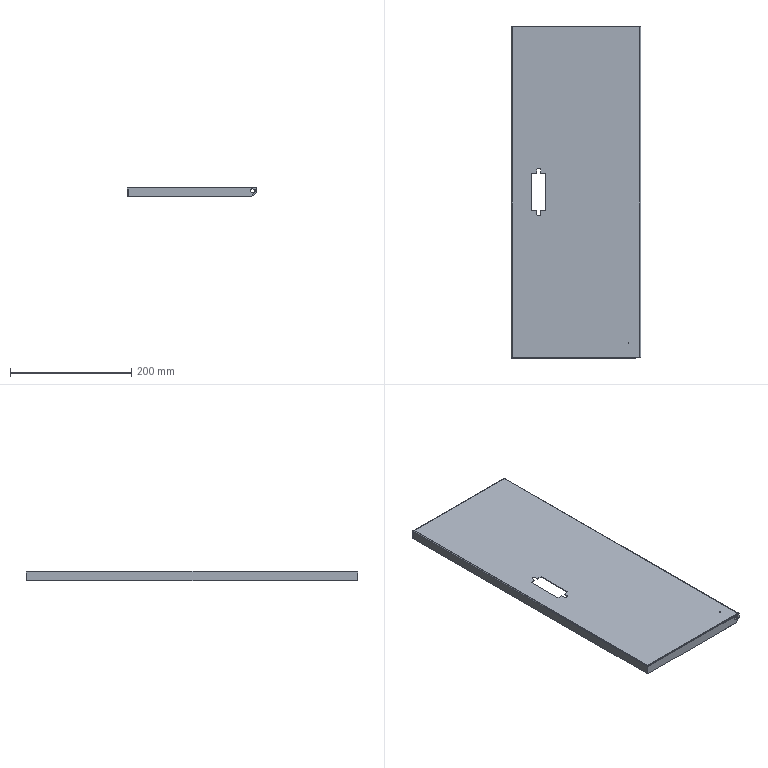Part | SolidWorks | features EdgeFlange 4, FlatPattern 1, ICE 1, SMBaseFlange 1, SheetMetal 1 | 1 solid | 70 faces | box 213 x 547 x 16 mm | volume 163711 mm3 | plane 52 | cylinder 18 | commonest cylinder face diameters 0.4 x5 2.8 x5 6.5 x4 1.6 x2 6.4 x2